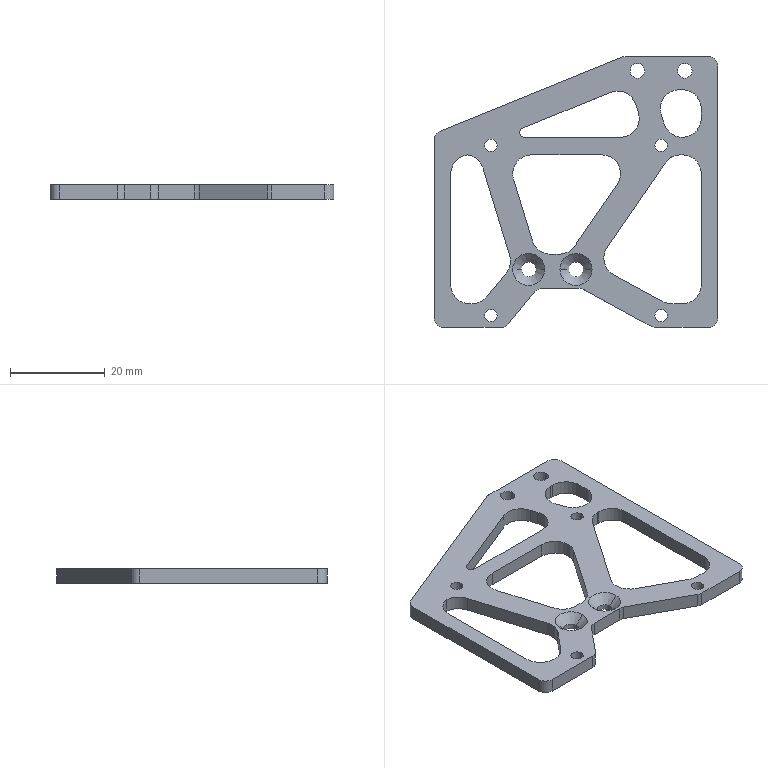Part | SolidWorks | features Fillet 3, RefAxis 2, RevCut 2, Extrusion 1, ICE 1 | 1 solid | 85 faces | box 60 x 57.271 x 3 mm | volume 4694 mm3 | cylinder 50 | plane 31 | cone 4 | commonest cylinder face diameters 8 x23 4 x9 2.6 x8 3.1 x8 2 x2